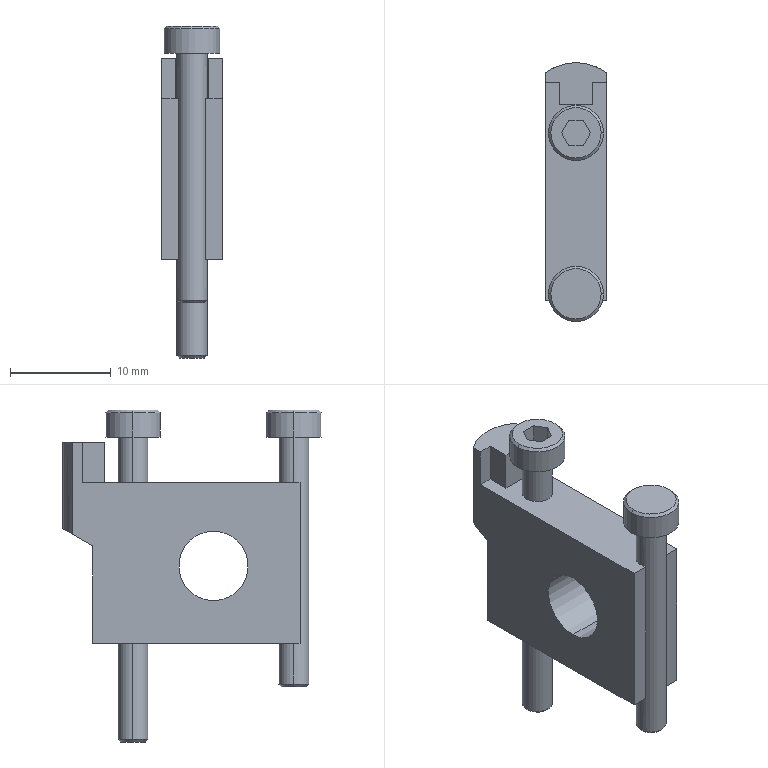Part | STEP file | AC10B-M5_AC3011A Spacer Interface(1) | 1 solid | 49 faces | box 6 x 25.75 x 33 mm | volume 2218 mm3 | plane 27 | cylinder 14 | cone 8 | commonest cylinder face diameters 3 x7 5.5 x4 6.9 x2 10 x1